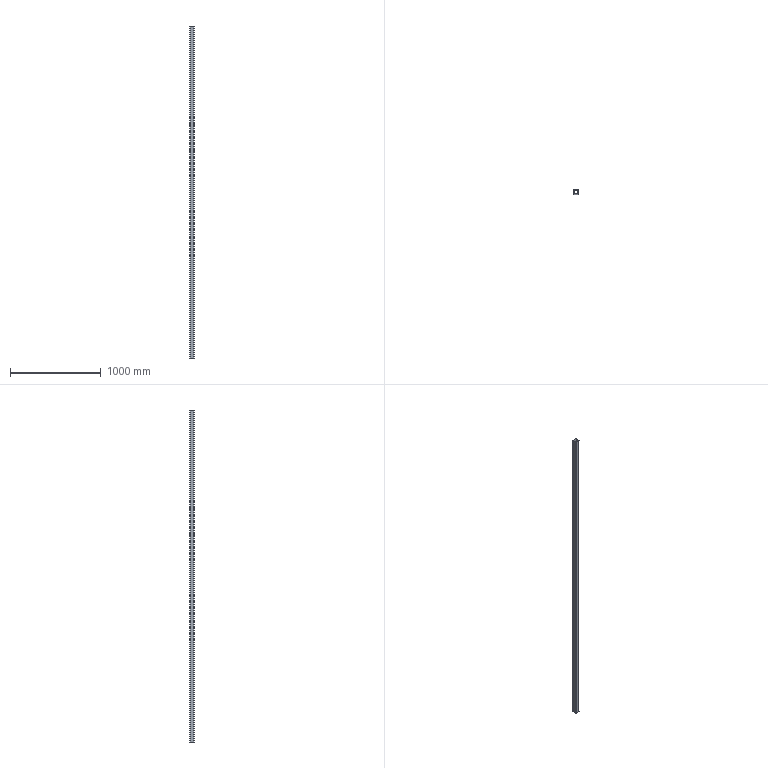Part | STEP file | Square steel 50×50×3650 | 1 solid | 18 faces | box 50 x 50 x 3650 mm | volume 2611204 mm3 | plane 10 | cylinder 8 | commonest cylinder face diameters 2 x4 10 x4
STEP:
#1=CARTESIAN_POINT('',(0.,0.,0.));
#2=DIRECTION('',(0.,0.,1.));
#3=DIRECTION('',(1.,0.,0.));
#4=AXIS2_PLACEMENT_3D('',#1,#2,#3);
#5=CARTESIAN_POINT('',(-25.,-20.,1825.));
#6=VERTEX_POINT('',#5);
#7=CARTESIAN_POINT('',(-20.,-25.,1825.));
#8=VERTEX_POINT('',#7);
#9=CARTESIAN_POINT('',(-20.,-20.,1825.));
#10=DIRECTION('',(0.,0.,1.));
#11=DIRECTION('',(1.,0.,0.));
#12=AXIS2_PLACEMENT_3D('',#9,#10,#11);
#13=CIRCLE('',#12,5.);
#14=CARTESIAN_POINT('',(-20.,-20.,1825.));
#15=DIRECTION('',(0.,0.,1.));
#16=DIRECTION('',(1.,0.,0.));
#17=AXIS2_PLACEMENT_3D('',#14,#15,#16);
#18=PLANE('',#17);
#19=CARTESIAN_POINT('',(0.,0.));
#20=DIRECTION('',(1.,0.));
#21=AXIS2_PLACEMENT_2D('',#19,#20);
#22=CIRCLE('',#21,5.);
#23=(GEOMETRIC_REPRESENTATION_CONTEXT(2)PARAMETRIC_REPRESENTATION_CONTEXT()REPRESENTATION_CONTEXT('',''));
#24=DEFINITIONAL_REPRESENTATION('',(#22),#23);
#25=PCURVE('',#18,#24);
#26=CARTESIAN_POINT('',(-20.,-20.,1825.));
#27=DIRECTION('',(0.,0.,-1.));
#28=DIRECTION('',(-1.,0.,0.));
#29=AXIS2_PLACEMENT_3D('',#26,#27,#28);
#30=CYLINDRICAL_SURFACE('',#29,5.);
#31=CARTESIAN_POINT('',(9.425,0.));
#32=DIRECTION('',(-1.,0.));
#33=VECTOR('',#32,1.);
#34=LINE('',#31,#33);
#35=(GEOMETRIC_REPRESENTATION_CONTEXT(2)PARAMETRIC_REPRESENTATION_CONTEXT()REPRESENTATION_CONTEXT('',''));
#36=DEFINITIONAL_REPRESENTATION('',(#34),#35);
#37=PCURVE('',#30,#36);
#38=SURFACE_CURVE('',#13,(#25,#37),.PCURVE_S1.);
#39=EDGE_CURVE('',#6,#8,#38,.T.);
#40=ORIENTED_EDGE('',*,*,#39,.T.);
#41=CARTESIAN_POINT('',(20.,-25.,1825.));
#42=VERTEX_POINT('',#41);
#43=CARTESIAN_POINT('',(-20.,-25.,1825.));
#44=DIRECTION('',(1.,0.,0.));
#45=VECTOR('',#44,1.);
#46=LINE('',#43,#45);
#47=CARTESIAN_POINT('',(0.,-5.));
#48=DIRECTION('',(1.,0.));
#49=VECTOR('',#48,1.);
#50=LINE('',#47,#49);
#51=(GEOMETRIC_REPRESENTATION_CONTEXT(2)PARAMETRIC_REPRESENTATION_CONTEXT()REPRESENTATION_CONTEXT('',''));
#52=DEFINITIONAL_REPRESENTATION('',(#50),#51);
#53=PCURVE('',#18,#52);
#54=CARTESIAN_POINT('',(-20.,-25.,1825.));
#55=DIRECTION('',(0.,1.,0.));
#56=DIRECTION('',(0.,0.,1.));
#57=AXIS2_PLACEMENT_3D('',#54,#55,#56);
#58=PLANE('',#57);
#59=CARTESIAN_POINT('',(0.,0.));
#60=DIRECTION('',(0.,1.));
#61=VECTOR('',#60,1.);
#62=LINE('',#59,#61);
#63=(GEOMETRIC_REPRESENTATION_CONTEXT(2)PARAMETRIC_REPRESENTATION_CONTEXT()REPRESENTATION_CONTEXT('',''));
#64=DEFINITIONAL_REPRESENTATION('',(#62),#63);
#65=PCURVE('',#58,#64);
#66=SURFACE_CURVE('',#46,(#53,#65),.PCURVE_S1.);
#67=EDGE_CURVE('',#8,#42,#66,.T.);
#68=ORIENTED_EDGE('',*,*,#67,.T.);
#69=CARTESIAN_POINT('',(25.,-20.,1825.));
#70=VERTEX_POINT('',#69);
#71=CARTESIAN_POINT('',(20.,-20.,1825.));
#72=DIRECTION('',(0.,0.,1.));
#73=DIRECTION('',(-1.,0.,0.));
#74=AXIS2_PLACEMENT_3D('',#71,#72,#73);
#75=CIRCLE('',#74,5.);
#76=CARTESIAN_POINT('',(40.,0.));
#77=DIRECTION('',(-1.,0.));
#78=AXIS2_PLACEMENT_2D('',#76,#77);
#79=CIRCLE('',#78,5.);
#80=(GEOMETRIC_REPRESENTATION_CONTEXT(2)PARAMETRIC_REPRESENTATION_CONTEXT()REPRESENTATION_CONTEXT('',''));
#81=DEFINITIONAL_REPRESENTATION('',(#79),#80);
#82=PCURVE('',#18,#81);
#83=CARTESIAN_POINT('',(20.,-20.,1825.));
#84=DIRECTION('',(0.,0.,-1.));
#85=DIRECTION('',(-1.,0.,0.));
#86=AXIS2_PLACEMENT_3D('',#83,#84,#85);
#87=CYLINDRICAL_SURFACE('',#86,5.);
#88=CARTESIAN_POINT('',(6.283,0.));
#89=DIRECTION('',(-1.,0.));
#90=VECTOR('',#89,1.);
#91=LINE('',#88,#90);
#92=(GEOMETRIC_REPRESENTATION_CONTEXT(2)PARAMETRIC_REPRESENTATION_CONTEXT()REPRESENTATION_CONTEXT('',''));
#93=DEFINITIONAL_REPRESENTATION('',(#91),#92);
#94=PCURVE('',#87,#93);
#95=SURFACE_CURVE('',#75,(#82,#94),.PCURVE_S1.);
#96=EDGE_CURVE('',#42,#70,#95,.T.);
#97=ORIENTED_EDGE('',*,*,#96,.T.);
#98=CARTESIAN_POINT('',(25.,20.,1825.));
#99=VERTEX_POINT('',#98);
#100=CARTESIAN_POINT('',(25.,20.,1825.));
#101=DIRECTION('',(0.,1.,0.));
#102=VECTOR('',#101,1.);
#103=LINE('',#100,#102);
#104=CARTESIAN_POINT('',(45.,40.));
#105=DIRECTION('',(0.,1.));
#106=VECTOR('',#105,1.);
#107=LINE('',#104,#106);
#108=(GEOMETRIC_REPRESENTATION_CONTEXT(2)PARAMETRIC_REPRESENTATION_CONTEXT()REPRESENTATION_CONTEXT('',''));
#109=DEFINITIONAL_REPRESENTATION('',(#107),#108);
#110=PCURVE('',#18,#109);
#111=CARTESIAN_POINT('',(25.,20.,1825.));
#112=DIRECTION('',(-1.,0.,0.));
#113=DIRECTION('',(0.,-1.,0.));
#114=AXIS2_PLACEMENT_3D('',#111,#112,#113);
#115=PLANE('',#114);
#116=CARTESIAN_POINT('',(0.,0.));
#117=DIRECTION('',(-1.,0.));
#118=VECTOR('',#117,1.);
#119=LINE('',#116,#118);
#120=(GEOMETRIC_REPRESENTATION_CONTEXT(2)PARAMETRIC_REPRESENTATION_CONTEXT()REPRESENTATION_CONTEXT('',''));
#121=DEFINITIONAL_REPRESENTATION('',(#119),#120);
#122=PCURVE('',#115,#121);
#123=SURFACE_CURVE('',#103,(#110,#122),.PCURVE_S1.);
#124=EDGE_CURVE('',#70,#99,#123,.T.);
#125=ORIENTED_EDGE('',*,*,#124,.T.);
#126=CARTESIAN_POINT('',(20.,25.,1825.));
#127=VERTEX_POINT('',#126);
#128=CARTESIAN_POINT('',(20.,20.,1825.));
#129=DIRECTION('',(0.,0.,1.));
#130=DIRECTION('',(1.,0.,0.));
#131=AXIS2_PLACEMENT_3D('',#128,#129,#130);
#132=CIRCLE('',#131,5.);
#133=CARTESIAN_POINT('',(40.,40.));
#134=DIRECTION('',(1.,0.));
#135=AXIS2_PLACEMENT_2D('',#133,#134);
#136=CIRCLE('',#135,5.);
#137=(GEOMETRIC_REPRESENTATION_CONTEXT(2)PARAMETRIC_REPRESENTATION_CONTEXT()REPRESENTATION_CONTEXT('',''));
#138=DEFINITIONAL_REPRESENTATION('',(#136),#137);
#139=PCURVE('',#18,#138);
#140=CARTESIAN_POINT('',(20.,20.,1825.));
#141=DIRECTION('',(0.,0.,-1.));
#142=DIRECTION('',(-1.,0.,0.));
#143=AXIS2_PLACEMENT_3D('',#140,#141,#142);
#144=CYLINDRICAL_SURFACE('',#143,5.);
#145=CARTESIAN_POINT('',(3.142,0.));
#146=DIRECTION('',(-1.,0.));
#147=VECTOR('',#146,1.);
#148=LINE('',#145,#147);
#149=(GEOMETRIC_REPRESENTATION_CONTEXT(2)PARAMETRIC_REPRESENTATION_CONTEXT()REPRESENTATION_CONTEXT('',''));
#150=DEFINITIONAL_REPRESENTATION('',(#148),#149);
#151=PCURVE('',#144,#150);
#152=SURFACE_CURVE('',#132,(#139,#151),.PCURVE_S1.);
#153=EDGE_CURVE('',#99,#127,#152,.T.);
#154=ORIENTED_EDGE('',*,*,#153,.T.);
#155=CARTESIAN_POINT('',(-20.,25.,1825.));
#156=VERTEX_POINT('',#155);
#157=CARTESIAN_POINT('',(-20.,25.,1825.));
#158=DIRECTION('',(-1.,0.,0.));
#159=VECTOR('',#158,1.);
#160=LINE('',#157,#159);
#161=CARTESIAN_POINT('',(0.,45.));
#162=DIRECTION('',(-1.,0.));
#163=VECTOR('',#162,1.);
#164=LINE('',#161,#163);
#165=(GEOMETRIC_REPRESENTATION_CONTEXT(2)PARAMETRIC_REPRESENTATION_CONTEXT()REPRESENTATION_CONTEXT('',''));
#166=DEFINITIONAL_REPRESENTATION('',(#164),#165);
#167=PCURVE('',#18,#166);
#168=CARTESIAN_POINT('',(-20.,25.,1825.));
#169=DIRECTION('',(0.,-1.,0.));
#170=DIRECTION('',(0.,0.,-1.));
#171=AXIS2_PLACEMENT_3D('',#168,#169,#170);
#172=PLANE('',#171);
#173=CARTESIAN_POINT('',(0.,0.));
#174=DIRECTION('',(0.,-1.));
#175=VECTOR('',#174,1.);
#176=LINE('',#173,#175);
#177=(GEOMETRIC_REPRESENTATION_CONTEXT(2)PARAMETRIC_REPRESENTATION_CONTEXT()REPRESENTATION_CONTEXT('',''));
#178=DEFINITIONAL_REPRESENTATION('',(#176),#177);
#179=PCURVE('',#172,#178);
#180=SURFACE_CURVE('',#160,(#167,#179),.PCURVE_S1.);
#181=EDGE_CURVE('',#127,#156,#180,.T.);
#182=ORIENTED_EDGE('',*,*,#181,.T.);
#183=CARTESIAN_POINT('',(-25.,20.,1825.));
#184=VERTEX_POINT('',#183);
#185=CARTESIAN_POINT('',(-20.,20.,1825.));
#186=DIRECTION('',(0.,0.,1.));
#187=DIRECTION('',(-1.,0.,0.));
#188=AXIS2_PLACEMENT_3D('',#185,#186,#187);
#189=CIRCLE('',#188,5.);
#190=CARTESIAN_POINT('',(0.,40.));
#191=DIRECTION('',(-1.,0.));
#192=AXIS2_PLACEMENT_2D('',#190,#191);
#193=CIRCLE('',#192,5.);
#194=(GEOMETRIC_REPRESENTATION_CONTEXT(2)PARAMETRIC_REPRESENTATION_CONTEXT()REPRESENTATION_CONTEXT('',''));
#195=DEFINITIONAL_REPRESENTATION('',(#193),#194);
#196=PCURVE('',#18,#195);
#197=CARTESIAN_POINT('',(-20.,20.,1825.));
#198=DIRECTION('',(0.,0.,-1.));
#199=DIRECTION('',(-1.,0.,0.));
#200=AXIS2_PLACEMENT_3D('',#197,#198,#199);
#201=CYLINDRICAL_SURFACE('',#200,5.);
#202=CARTESIAN_POINT('',(6.283,0.));
#203=DIRECTION('',(-1.,0.));
#204=VECTOR('',#203,1.);
#205=LINE('',#202,#204);
#206=(GEOMETRIC_REPRESENTATION_CONTEXT(2)PARAMETRIC_REPRESENTATION_CONTEXT()REPRESENTATION_CONTEXT('',''));
#207=DEFINITIONAL_REPRESENTATION('',(#205),#206);
#208=PCURVE('',#201,#207);
#209=SURFACE_CURVE('',#189,(#196,#208),.PCURVE_S1.);
#210=EDGE_CURVE('',#156,#184,#209,.T.);
#211=ORIENTED_EDGE('',*,*,#210,.T.);
#212=CARTESIAN_POINT('',(-25.,20.,1825.));
#213=DIRECTION('',(0.,-1.,0.));
#214=VECTOR('',#213,1.);
#215=LINE('',#212,#214);
#216=CARTESIAN_POINT('',(-5.,40.));
#217=DIRECTION('',(0.,-1.));
#218=VECTOR('',#217,1.);
#219=LINE('',#216,#218);
#220=(GEOMETRIC_REPRESENTATION_CONTEXT(2)PARAMETRIC_REPRESENTATION_CONTEXT()REPRESENTATION_CONTEXT('',''));
#221=DEFINITIONAL_REPRESENTATION('',(#219),#220);
#222=PCURVE('',#18,#221);
#223=CARTESIAN_POINT('',(-25.,20.,1825.));
#224=DIRECTION('',(1.,0.,0.));
#225=DIRECTION('',(0.,1.,0.));
#226=AXIS2_PLACEMENT_3D('',#223,#224,#225);
#227=PLANE('',#226);
#228=CARTESIAN_POINT('',(0.,0.));
#229=DIRECTION('',(-1.,0.));
#230=VECTOR('',#229,1.);
#231=LINE('',#228,#230);
#232=(GEOMETRIC_REPRESENTATION_CONTEXT(2)PARAMETRIC_REPRESENTATION_CONTEXT()REPRESENTATION_CONTEXT('',''));
#233=DEFINITIONAL_REPRESENTATION('',(#231),#232);
#234=PCURVE('',#227,#233);
#235=SURFACE_CURVE('',#215,(#222,#234),.PCURVE_S1.);
#236=EDGE_CURVE('',#184,#6,#235,.T.);
#237=ORIENTED_EDGE('',*,*,#236,.T.);
#238=EDGE_LOOP('',(#40,#68,#97,#125,#154,#182,#211,#237));
#239=FACE_BOUND('',#238,.T.);
#240=CARTESIAN_POINT('',(-21.,20.,1825.));
#241=VERTEX_POINT('',#240);
#242=CARTESIAN_POINT('',(-21.,-20.,1825.));
#243=VERTEX_POINT('',#242);
#244=CARTESIAN_POINT('',(-21.,20.,1825.));
#245=DIRECTION('',(0.,-1.,0.));
#246=VECTOR('',#245,1.);
#247=LINE('',#244,#246);
#248=CARTESIAN_POINT('',(-1.,40.));
#249=DIRECTION('',(0.,-1.));
#250=VECTOR('',#249,1.);
#251=LINE('',#248,#250);
#252=(GEOMETRIC_REPRESENTATION_CONTEXT(2)PARAMETRIC_REPRESENTATION_CONTEXT()REPRESENTATION_CONTEXT('',''));
#253=DEFINITIONAL_REPRESENTATION('',(#251),#252);
#254=PCURVE('',#18,#253);
#255=CARTESIAN_POINT('',(-21.,20.,1825.));
#256=DIRECTION('',(1.,0.,0.));
#257=DIRECTION('',(0.,1.,0.));
#258=AXIS2_PLACEMENT_3D('',#255,#256,#257);
#259=PLANE('',#258);
#260=CARTESIAN_POINT('',(0.,0.));
#261=DIRECTION('',(-1.,0.));
#262=VECTOR('',#261,1.);
#263=LINE('',#260,#262);
#264=(GEOMETRIC_REPRESENTATION_CONTEXT(2)PARAMETRIC_REPRESENTATION_CONTEXT()REPRESENTATION_CONTEXT('',''));
#265=DEFINITIONAL_REPRESENTATION('',(#263),#264);
#266=PCURVE('',#259,#265);
#267=SURFACE_CURVE('',#247,(#254,#266),.PCURVE_S1.);
#268=EDGE_CURVE('',#241,#243,#267,.T.);
#269=ORIENTED_EDGE('',*,*,#268,.F.);
#270=CARTESIAN_POINT('',(-20.,21.,1825.));
#271=VERTEX_POINT('',#270);
#272=CARTESIAN_POINT('',(-20.,20.,1825.));
#273=DIRECTION('',(0.,0.,1.));
#274=DIRECTION('',(-1.,0.,0.));
#275=AXIS2_PLACEMENT_3D('',#272,#273,#274);
#276=CIRCLE('',#275,1.);
#277=CARTESIAN_POINT('',(0.,40.));
#278=DIRECTION('',(-1.,0.));
#279=AXIS2_PLACEMENT_2D('',#277,#278);
#280=CIRCLE('',#279,1.);
#281=(GEOMETRIC_REPRESENTATION_CONTEXT(2)PARAMETRIC_REPRESENTATION_CONTEXT()REPRESENTATION_CONTEXT('',''));
#282=DEFINITIONAL_REPRESENTATION('',(#280),#281);
#283=PCURVE('',#18,#282);
#284=CARTESIAN_POINT('',(-20.,20.,1825.));
#285=DIRECTION('',(0.,0.,-1.));
#286=DIRECTION('',(-1.,0.,0.));
#287=AXIS2_PLACEMENT_3D('',#284,#285,#286);
#288=CYLINDRICAL_SURFACE('',#287,1.);
#289=CARTESIAN_POINT('',(6.283,0.));
#290=DIRECTION('',(-1.,0.));
#291=VECTOR('',#290,1.);
#292=LINE('',#289,#291);
#293=(GEOMETRIC_REPRESENTATION_CONTEXT(2)PARAMETRIC_REPRESENTATION_CONTEXT()REPRESENTATION_CONTEXT('',''));
#294=DEFINITIONAL_REPRESENTATION('',(#292),#293);
#295=PCURVE('',#288,#294);
#296=SURFACE_CURVE('',#276,(#283,#295),.PCURVE_S1.);
#297=EDGE_CURVE('',#271,#241,#296,.T.);
#298=ORIENTED_EDGE('',*,*,#297,.F.);
#299=CARTESIAN_POINT('',(20.,21.,1825.));
#300=VERTEX_POINT('',#299);
#301=CARTESIAN_POINT('',(-20.,21.,1825.));
#302=DIRECTION('',(-1.,0.,0.));
#303=VECTOR('',#302,1.);
#304=LINE('',#301,#303);
#305=CARTESIAN_POINT('',(0.,41.));
#306=DIRECTION('',(-1.,0.));
#307=VECTOR('',#306,1.);
#308=LINE('',#305,#307);
#309=(GEOMETRIC_REPRESENTATION_CONTEXT(2)PARAMETRIC_REPRESENTATION_CONTEXT()REPRESENTATION_CONTEXT('',''));
#310=DEFINITIONAL_REPRESENTATION('',(#308),#309);
#311=PCURVE('',#18,#310);
#312=CARTESIAN_POINT('',(-20.,21.,1825.));
#313=DIRECTION('',(0.,-1.,0.));
#314=DIRECTION('',(0.,0.,-1.));
#315=AXIS2_PLACEMENT_3D('',#312,#313,#314);
#316=PLANE('',#315);
#317=CARTESIAN_POINT('',(0.,0.));
#318=DIRECTION('',(0.,-1.));
#319=VECTOR('',#318,1.);
#320=LINE('',#317,#319);
#321=(GEOMETRIC_REPRESENTATION_CONTEXT(2)PARAMETRIC_REPRESENTATION_CONTEXT()REPRESENTATION_CONTEXT('',''));
#322=DEFINITIONAL_REPRESENTATION('',(#320),#321);
#323=PCURVE('',#316,#322);
#324=SURFACE_CURVE('',#304,(#311,#323),.PCURVE_S1.);
#325=EDGE_CURVE('',#300,#271,#324,.T.);
#326=ORIENTED_EDGE('',*,*,#325,.F.);
#327=CARTESIAN_POINT('',(21.,20.,1825.));
#328=VERTEX_POINT('',#327);
#329=CARTESIAN_POINT('',(20.,20.,1825.));
#330=DIRECTION('',(0.,0.,1.));
#331=DIRECTION('',(1.,0.,0.));
#332=AXIS2_PLACEMENT_3D('',#329,#330,#331);
#333=CIRCLE('',#332,1.);
#334=CARTESIAN_POINT('',(40.,40.));
#335=DIRECTION('',(1.,0.));
#336=AXIS2_PLACEMENT_2D('',#334,#335);
#337=CIRCLE('',#336,1.);
#338=(GEOMETRIC_REPRESENTATION_CONTEXT(2)PARAMETRIC_REPRESENTATION_CONTEXT()REPRESENTATION_CONTEXT('',''));
#339=DEFINITIONAL_REPRESENTATION('',(#337),#338);
#340=PCURVE('',#18,#339);
#341=CARTESIAN_POINT('',(20.,20.,1825.));
#342=DIRECTION('',(0.,0.,-1.));
#343=DIRECTION('',(-1.,0.,0.));
#344=AXIS2_PLACEMENT_3D('',#341,#342,#343);
#345=CYLINDRICAL_SURFACE('',#344,1.);
#346=CARTESIAN_POINT('',(3.142,0.));
#347=DIRECTION('',(-1.,0.));
#348=VECTOR('',#347,1.);
#349=LINE('',#346,#348);
#350=(GEOMETRIC_REPRESENTATION_CONTEXT(2)PARAMETRIC_REPRESENTATION_CONTEXT()REPRESENTATION_CONTEXT('',''));
#351=DEFINITIONAL_REPRESENTATION('',(#349),#350);
#352=PCURVE('',#345,#351);
#353=SURFACE_CURVE('',#333,(#340,#352),.PCURVE_S1.);
#354=EDGE_CURVE('',#328,#300,#353,.T.);
#355=ORIENTED_EDGE('',*,*,#354,.F.);
#356=CARTESIAN_POINT('',(21.,-20.,1825.));
#357=VERTEX_POINT('',#356);
#358=CARTESIAN_POINT('',(21.,20.,1825.));
#359=DIRECTION('',(0.,1.,0.));
#360=VECTOR('',#359,1.);
#361=LINE('',#358,#360);
#362=CARTESIAN_POINT('',(41.,40.));
#363=DIRECTION('',(0.,1.));
#364=VECTOR('',#363,1.);
#365=LINE('',#362,#364);
#366=(GEOMETRIC_REPRESENTATION_CONTEXT(2)PARAMETRIC_REPRESENTATION_CONTEXT()REPRESENTATION_CONTEXT('',''));
#367=DEFINITIONAL_REPRESENTATION('',(#365),#366);
#368=PCURVE('',#18,#367);
#369=CARTESIAN_POINT('',(21.,20.,1825.));
#370=DIRECTION('',(-1.,0.,0.));
#371=DIRECTION('',(0.,0.,1.));
#372=AXIS2_PLACEMENT_3D('',#369,#370,#371);
#373=PLANE('',#372);
#374=CARTESIAN_POINT('',(0.,0.));
#375=DIRECTION('',(0.,1.));
#376=VECTOR('',#375,1.);
#377=LINE('',#374,#376);
#378=(GEOMETRIC_REPRESENTATION_CONTEXT(2)PARAMETRIC_REPRESENTATION_CONTEXT()REPRESENTATION_CONTEXT('',''));
#379=DEFINITIONAL_REPRESENTATION('',(#377),#378);
#380=PCURVE('',#373,#379);
#381=SURFACE_CURVE('',#361,(#368,#380),.PCURVE_S1.);
#382=EDGE_CURVE('',#357,#328,#381,.T.);
#383=ORIENTED_EDGE('',*,*,#382,.F.);
#384=CARTESIAN_POINT('',(20.,-21.,1825.));
#385=VERTEX_POINT('',#384);
#386=CARTESIAN_POINT('',(20.,-20.,1825.));
#387=DIRECTION('',(0.,0.,1.));
#388=DIRECTION('',(-1.,0.,0.));
#389=AXIS2_PLACEMENT_3D('',#386,#387,#388);
#390=CIRCLE('',#389,1.);
#391=CARTESIAN_POINT('',(40.,0.));
#392=DIRECTION('',(-1.,0.));
#393=AXIS2_PLACEMENT_2D('',#391,#392);
#394=CIRCLE('',#393,1.);
#395=(GEOMETRIC_REPRESENTATION_CONTEXT(2)PARAMETRIC_REPRESENTATION_CONTEXT()REPRESENTATION_CONTEXT('',''));
#396=DEFINITIONAL_REPRESENTATION('',(#394),#395);
#397=PCURVE('',#18,#396);
#398=CARTESIAN_POINT('',(20.,-20.,1825.));
#399=DIRECTION('',(0.,0.,-1.));
#400=DIRECTION('',(-1.,0.,0.));
#401=AXIS2_PLACEMENT_3D('',#398,#399,#400);
#402=CYLINDRICAL_SURFACE('',#401,1.);
#403=CARTESIAN_POINT('',(6.283,0.));
#404=DIRECTION('',(-1.,0.));
#405=VECTOR('',#404,1.);
#406=LINE('',#403,#405);
#407=(GEOMETRIC_REPRESENTATION_CONTEXT(2)PARAMETRIC_REPRESENTATION_CONTEXT()REPRESENTATION_CONTEXT('',''));
#408=DEFINITIONAL_REPRESENTATION('',(#406),#407);
#409=PCURVE('',#402,#408);
#410=SURFACE_CURVE('',#390,(#397,#409),.PCURVE_S1.);
#411=EDGE_CURVE('',#385,#357,#410,.T.);
#412=ORIENTED_EDGE('',*,*,#411,.F.);
#413=CARTESIAN_POINT('',(-20.,-21.,1825.));
#414=VERTEX_POINT('',#413);
#415=CARTESIAN_POINT('',(-20.,-21.,1825.));
#416=DIRECTION('',(1.,0.,0.));
#417=VECTOR('',#416,1.);
#418=LINE('',#415,#417);
#419=CARTESIAN_POINT('',(0.,-1.));
#420=DIRECTION('',(1.,0.));
#421=VECTOR('',#420,1.);
#422=LINE('',#419,#421);
#423=(GEOMETRIC_REPRESENTATION_CONTEXT(2)PARAMETRIC_REPRESENTATION_CONTEXT()REPRESENTATION_CONTEXT('',''));
#424=DEFINITIONAL_REPRESENTATION('',(#422),#423);
#425=PCURVE('',#18,#424);
#426=CARTESIAN_POINT('',(-20.,-21.,1825.));
#427=DIRECTION('',(0.,1.,0.));
#428=DIRECTION('',(0.,0.,1.));
#429=AXIS2_PLACEMENT_3D('',#426,#427,#428);
#430=PLANE('',#429);
#431=CARTESIAN_POINT('',(0.,0.));
#432=DIRECTION('',(0.,1.));
#433=VECTOR('',#432,1.);
#434=LINE('',#431,#433);
#435=(GEOMETRIC_REPRESENTATION_CONTEXT(2)PARAMETRIC_REPRESENTATION_CONTEXT()REPRESENTATION_CONTEXT('',''));
#436=DEFINITIONAL_REPRESENTATION('',(#434),#435);
#437=PCURVE('',#430,#436);
#438=SURFACE_CURVE('',#418,(#425,#437),.PCURVE_S1.);
#439=EDGE_CURVE('',#414,#385,#438,.T.);
#440=ORIENTED_EDGE('',*,*,#439,.F.);
#441=CARTESIAN_POINT('',(-20.,-20.,1825.));
#442=DIRECTION('',(0.,0.,1.));
#443=DIRECTION('',(1.,0.,0.));
#444=AXIS2_PLACEMENT_3D('',#441,#442,#443);
#445=CIRCLE('',#444,1.);
#446=CARTESIAN_POINT('',(0.,0.));
#447=DIRECTION('',(1.,0.));
#448=AXIS2_PLACEMENT_2D('',#446,#447);
#449=CIRCLE('',#448,1.);
#450=(GEOMETRIC_REPRESENTATION_CONTEXT(2)PARAMETRIC_REPRESENTATION_CONTEXT()REPRESENTATION_CONTEXT('',''));
#451=DEFINITIONAL_REPRESENTATION('',(#449),#450);
#452=PCURVE('',#18,#451);
#453=CARTESIAN_POINT('',(-20.,-20.,1825.));
#454=DIRECTION('',(0.,0.,-1.));
#455=DIRECTION('',(-1.,0.,0.));
#456=AXIS2_PLACEMENT_3D('',#453,#454,#455);
#457=CYLINDRICAL_SURFACE('',#456,1.);
#458=CARTESIAN_POINT('',(9.425,0.));
#459=DIRECTION('',(-1.,0.));
#460=VECTOR('',#459,1.);
#461=LINE('',#458,#460);
#462=(GEOMETRIC_REPRESENTATION_CONTEXT(2)PARAMETRIC_REPRESENTATION_CONTEXT()REPRESENTATION_CONTEXT('',''));
#463=DEFINITIONAL_REPRESENTATION('',(#461),#462);
#464=PCURVE('',#457,#463);
#465=SURFACE_CURVE('',#445,(#452,#464),.PCURVE_S1.);
#466=EDGE_CURVE('',#243,#414,#465,.T.);
#467=ORIENTED_EDGE('',*,*,#466,.F.);
#468=EDGE_LOOP('',(#269,#298,#326,#355,#383,#412,#440,#467));
#469=FACE_BOUND('',#468,.T.);
#470=ADVANCED_FACE('',(#239,#469),#18,.T.);
#471=CARTESIAN_POINT('',(-25.,-20.,-1825.));
#472=VERTEX_POINT('',#471);
#473=CARTESIAN_POINT('',(-20.,-25.,-1825.));
#474=VERTEX_POINT('',#473);
#475=CARTESIAN_POINT('',(-20.,-20.,-1825.));
#476=DIRECTION('',(0.,0.,1.));
#477=DIRECTION('',(1.,0.,0.));
#478=AXIS2_PLACEMENT_3D('',#475,#476,#477);
#479=CIRCLE('',#478,5.);
#480=CARTESIAN_POINT('',(-20.,-20.,-1825.));
#481=DIRECTION('',(0.,0.,1.));
#482=DIRECTION('',(1.,0.,0.));
#483=AXIS2_PLACEMENT_3D('',#480,#481,#482);
#484=PLANE('',#483);
#485=CARTESIAN_POINT('',(0.,0.));
#486=DIRECTION('',(1.,0.));
#487=AXIS2_PLACEMENT_2D('',#485,#486);
#488=CIRCLE('',#487,5.);
#489=(GEOMETRIC_REPRESENTATION_CONTEXT(2)PARAMETRIC_REPRESENTATION_CONTEXT()REPRESENTATION_CONTEXT('',''));
#490=DEFINITIONAL_REPRESENTATION('',(#488),#489);
#491=PCURVE('',#484,#490);
#492=CARTESIAN_POINT('',(9.425,3650.));
#493=DIRECTION('',(-1.,0.));
#494=VECTOR('',#493,1.);
#495=LINE('',#492,#494);
#496=(GEOMETRIC_REPRESENTATION_CONTEXT(2)PARAMETRIC_REPRESENTATION_CONTEXT()REPRESENTATION_CONTEXT('',''));
#497=DEFINITIONAL_REPRESENTATION('',(#495),#496);
#498=PCURVE('',#30,#497);
#499=SURFACE_CURVE('',#479,(#491,#498),.PCURVE_S1.);
#500=EDGE_CURVE('',#472,#474,#499,.T.);
#501=ORIENTED_EDGE('',*,*,#500,.F.);
#502=CARTESIAN_POINT('',(-25.,20.,-1825.));
#503=VERTEX_POINT('',#502);
#504=CARTESIAN_POINT('',(-25.,20.,-1825.));
#505=DIRECTION('',(0.,-1.,0.));
#506=VECTOR('',#505,1.);
#507=LINE('',#504,#506);
#508=CARTESIAN_POINT('',(-5.,40.));
#509=DIRECTION('',(0.,-1.));
#510=VECTOR('',#509,1.);
#511=LINE('',#508,#510);
#512=(GEOMETRIC_REPRESENTATION_CONTEXT(2)PARAMETRIC_REPRESENTATION_CONTEXT()REPRESENTATION_CONTEXT('',''));
#513=DEFINITIONAL_REPRESENTATION('',(#511),#512);
#514=PCURVE('',#484,#513);
#515=CARTESIAN_POINT('',(0.,-3650.));
#516=DIRECTION('',(-1.,0.));
#517=VECTOR('',#516,1.);
#518=LINE('',#515,#517);
#519=(GEOMETRIC_REPRESENTATION_CONTEXT(2)PARAMETRIC_REPRESENTATION_CONTEXT()REPRESENTATION_CONTEXT('',''));
#520=DEFINITIONAL_REPRESENTATION('',(#518),#519);
#521=PCURVE('',#227,#520);
#522=SURFACE_CURVE('',#507,(#514,#521),.PCURVE_S1.);
#523=EDGE_CURVE('',#503,#472,#522,.T.);
#524=ORIENTED_EDGE('',*,*,#523,.F.);
#525=CARTESIAN_POINT('',(-20.,25.,-1825.));
#526=VERTEX_POINT('',#525);
#527=CARTESIAN_POINT('',(-20.,20.,-1825.));
#528=DIRECTION('',(0.,0.,1.));
#529=DIRECTION('',(-1.,0.,0.));
#530=AXIS2_PLACEMENT_3D('',#527,#528,#529);
#531=CIRCLE('',#530,5.);
#532=CARTESIAN_POINT('',(0.,40.));
#533=DIRECTION('',(-1.,0.));
#534=AXIS2_PLACEMENT_2D('',#532,#533);
#535=CIRCLE('',#534,5.);
#536=(GEOMETRIC_REPRESENTATION_CONTEXT(2)PARAMETRIC_REPRESENTATION_CONTEXT()REPRESENTATION_CONTEXT('',''));
#537=DEFINITIONAL_REPRESENTATION('',(#535),#536);
#538=PCURVE('',#484,#537);
#539=CARTESIAN_POINT('',(6.283,3650.));
#540=DIRECTION('',(-1.,0.));
#541=VECTOR('',#540,1.);
#542=LINE('',#539,#541);
#543=(GEOMETRIC_REPRESENTATION_CONTEXT(2)PARAMETRIC_REPRESENTATION_CONTEXT()REPRESENTATION_CONTEXT('',''));
#544=DEFINITIONAL_REPRESENTATION('',(#542),#543);
#545=PCURVE('',#201,#544);
#546=SURFACE_CURVE('',#531,(#538,#545),.PCURVE_S1.);
#547=EDGE_CURVE('',#526,#503,#546,.T.);
#548=ORIENTED_EDGE('',*,*,#547,.F.);
#549=CARTESIAN_POINT('',(20.,25.,-1825.));
#550=VERTEX_POINT('',#549);
#551=CARTESIAN_POINT('',(-20.,25.,-1825.));
#552=DIRECTION('',(-1.,0.,0.));
#553=VECTOR('',#552,1.);
#554=LINE('',#551,#553);
#555=CARTESIAN_POINT('',(0.,45.));
#556=DIRECTION('',(-1.,0.));
#557=VECTOR('',#556,1.);
#558=LINE('',#555,#557);
#559=(GEOMETRIC_REPRESENTATION_CONTEXT(2)PARAMETRIC_REPRESENTATION_CONTEXT()REPRESENTATION_CONTEXT('',''));
#560=DEFINITIONAL_REPRESENTATION('',(#558),#559);
#561=PCURVE('',#484,#560);
#562=CARTESIAN_POINT('',(3650.,0.));
#563=DIRECTION('',(0.,-1.));
#564=VECTOR('',#563,1.);
#565=LINE('',#562,#564);
#566=(GEOMETRIC_REPRESENTATION_CONTEXT(2)PARAMETRIC_REPRESENTATION_CONTEXT()REPRESENTATION_CONTEXT('',''));
#567=DEFINITIONAL_REPRESENTATION('',(#565),#566);
#568=PCURVE('',#172,#567);
#569=SURFACE_CURVE('',#554,(#561,#568),.PCURVE_S1.);
#570=EDGE_CURVE('',#550,#526,#569,.T.);
#571=ORIENTED_EDGE('',*,*,#570,.F.);
#572=CARTESIAN_POINT('',(25.,20.,-1825.));
#573=VERTEX_POINT('',#572);
#574=CARTESIAN_POINT('',(20.,20.,-1825.));
#575=DIRECTION('',(0.,0.,1.));
#576=DIRECTION('',(1.,0.,0.));
#577=AXIS2_PLACEMENT_3D('',#574,#575,#576);
#578=CIRCLE('',#577,5.);
#579=CARTESIAN_POINT('',(40.,40.));
#580=DIRECTION('',(1.,0.));
#581=AXIS2_PLACEMENT_2D('',#579,#580);
#582=CIRCLE('',#581,5.);
#583=(GEOMETRIC_REPRESENTATION_CONTEXT(2)PARAMETRIC_REPRESENTATION_CONTEXT()REPRESENTATION_CONTEXT('',''));
#584=DEFINITIONAL_REPRESENTATION('',(#582),#583);
#585=PCURVE('',#484,#584);
#586=CARTESIAN_POINT('',(3.142,3650.));
#587=DIRECTION('',(-1.,0.));
#588=VECTOR('',#587,1.);
#589=LINE('',#586,#588);
#590=(GEOMETRIC_REPRESENTATION_CONTEXT(2)PARAMETRIC_REPRESENTATION_CONTEXT()REPRESENTATION_CONTEXT('',''));
#591=DEFINITIONAL_REPRESENTATION('',(#589),#590);
#592=PCURVE('',#144,#591);
#593=SURFACE_CURVE('',#578,(#585,#592),.PCURVE_S1.);
#594=EDGE_CURVE('',#573,#550,#593,.T.);
#595=ORIENTED_EDGE('',*,*,#594,.F.);
#596=CARTESIAN_POINT('',(25.,-20.,-1825.));
#597=VERTEX_POINT('',#596);
#598=CARTESIAN_POINT('',(25.,20.,-1825.));
#599=DIRECTION('',(0.,1.,0.));
#600=VECTOR('',#599,1.);
#601=LINE('',#598,#600);
#602=CARTESIAN_POINT('',(45.,40.));
#603=DIRECTION('',(0.,1.));
#604=VECTOR('',#603,1.);
#605=LINE('',#602,#604);
#606=(GEOMETRIC_REPRESENTATION_CONTEXT(2)PARAMETRIC_REPRESENTATION_CONTEXT()REPRESENTATION_CONTEXT('',''));
#607=DEFINITIONAL_REPRESENTATION('',(#605),#606);
#608=PCURVE('',#484,#607);
#609=CARTESIAN_POINT('',(0.,-3650.));
#610=DIRECTION('',(-1.,0.));
#611=VECTOR('',#610,1.);
#612=LINE('',#609,#611);
#613=(GEOMETRIC_REPRESENTATION_CONTEXT(2)PARAMETRIC_REPRESENTATION_CONTEXT()REPRESENTATION_CONTEXT('',''));
#614=DEFINITIONAL_REPRESENTATION('',(#612),#613);
#615=PCURVE('',#115,#614);
#616=SURFACE_CURVE('',#601,(#608,#615),.PCURVE_S1.);
#617=EDGE_CURVE('',#597,#573,#616,.T.);
#618=ORIENTED_EDGE('',*,*,#617,.F.);
#619=CARTESIAN_POINT('',(20.,-25.,-1825.));
#620=VERTEX_POINT('',#619);
#621=CARTESIAN_POINT('',(20.,-20.,-1825.));
#622=DIRECTION('',(0.,0.,1.));
#623=DIRECTION('',(-1.,0.,0.));
#624=AXIS2_PLACEMENT_3D('',#621,#622,#623);
#625=CIRCLE('',#624,5.);
#626=CARTESIAN_POINT('',(40.,0.));
#627=DIRECTION('',(-1.,0.));
#628=AXIS2_PLACEMENT_2D('',#626,#627);
#629=CIRCLE('',#628,5.);
#630=(GEOMETRIC_REPRESENTATION_CONTEXT(2)PARAMETRIC_REPRESENTATION_CONTEXT()REPRESENTATION_CONTEXT('',''));
#631=DEFINITIONAL_REPRESENTATION('',(#629),#630);
#632=PCURVE('',#484,#631);
#633=CARTESIAN_POINT('',(6.283,3650.));
#634=DIRECTION('',(-1.,0.));
#635=VECTOR('',#634,1.);
#636=LINE('',#633,#635);
#637=(GEOMETRIC_REPRESENTATION_CONTEXT(2)PARAMETRIC_REPRESENTATION_CONTEXT()REPRESENTATION_CONTEXT('',''));
#638=DEFINITIONAL_REPRESENTATION('',(#636),#637);
#639=PCURVE('',#87,#638);
#640=SURFACE_CURVE('',#625,(#632,#639),.PCURVE_S1.);
#641=EDGE_CURVE('',#620,#597,#640,.T.);
#642=ORIENTED_EDGE('',*,*,#641,.F.);
#643=CARTESIAN_POINT('',(-20.,-25.,-1825.));
#644=DIRECTION('',(1.,0.,0.));
#645=VECTOR('',#644,1.);
#646=LINE('',#643,#645);
#647=CARTESIAN_POINT('',(0.,-5.));
#648=DIRECTION('',(1.,0.));
#649=VECTOR('',#648,1.);
#650=LINE('',#647,#649);
#651=(GEOMETRIC_REPRESENTATION_CONTEXT(2)PARAMETRIC_REPRESENTATION_CONTEXT()REPRESENTATION_CONTEXT('',''));
#652=DEFINITIONAL_REPRESENTATION('',(#650),#651);
#653=PCURVE('',#484,#652);
#654=CARTESIAN_POINT('',(-3650.,0.));
#655=DIRECTION('',(0.,1.));
#656=VECTOR('',#655,1.);
#657=LINE('',#654,#656);
#658=(GEOMETRIC_REPRESENTATION_CONTEXT(2)PARAMETRIC_REPRESENTATION_CONTEXT()REPRESENTATION_CONTEXT('',''));
#659=DEFINITIONAL_REPRESENTATION('',(#657),#658);
#660=PCURVE('',#58,#659);
#661=SURFACE_CURVE('',#646,(#653,#660),.PCURVE_S1.);
#662=EDGE_CURVE('',#474,#620,#661,.T.);
#663=ORIENTED_EDGE('',*,*,#662,.F.);
#664=EDGE_LOOP('',(#501,#524,#548,#571,#595,#618,#642,#663));
#665=FACE_BOUND('',#664,.T.);
#666=CARTESIAN_POINT('',(-20.,21.,-1825.));
#667=VERTEX_POINT('',#666);
#668=CARTESIAN_POINT('',(-21.,20.,-1825.));
#669=VERTEX_POINT('',#668);
#670=CARTESIAN_POINT('',(-20.,20.,-1825.));
#671=DIRECTION('',(0.,0.,1.));
#672=DIRECTION('',(-1.,0.,0.));
#673=AXIS2_PLACEMENT_3D('',#670,#671,#672);
#674=CIRCLE('',#673,1.);
#675=CARTESIAN_POINT('',(0.,40.));
#676=DIRECTION('',(-1.,0.));
#677=AXIS2_PLACEMENT_2D('',#675,#676);
#678=CIRCLE('',#677,1.);
#679=(GEOMETRIC_REPRESENTATION_CONTEXT(2)PARAMETRIC_REPRESENTATION_CONTEXT()REPRESENTATION_CONTEXT('',''));
#680=DEFINITIONAL_REPRESENTATION('',(#678),#679);
#681=PCURVE('',#484,#680);
#682=CARTESIAN_POINT('',(6.283,3650.));
#683=DIRECTION('',(-1.,0.));
#684=VECTOR('',#683,1.);
#685=LINE('',#682,#684);
#686=(GEOMETRIC_REPRESENTATION_CONTEXT(2)PARAMETRIC_REPRESENTATION_CONTEXT()REPRESENTATION_CONTEXT('',''));
#687=DEFINITIONAL_REPRESENTATION('',(#685),#686);
#688=PCURVE('',#288,#687);
#689=SURFACE_CURVE('',#674,(#681,#688),.PCURVE_S1.);
#690=EDGE_CURVE('',#667,#669,#689,.T.);
#691=ORIENTED_EDGE('',*,*,#690,.T.);
#692=CARTESIAN_POINT('',(-21.,-20.,-1825.));
#693=VERTEX_POINT('',#692);
#694=CARTESIAN_POINT('',(-21.,20.,-1825.));
#695=DIRECTION('',(0.,-1.,0.));
#696=VECTOR('',#695,1.);
#697=LINE('',#694,#696);
#698=CARTESIAN_POINT('',(-1.,40.));
#699=DIRECTION('',(0.,-1.));
#700=VECTOR('',#699,1.);
#701=LINE('',#698,#700);
#702=(GEOMETRIC_REPRESENTATION_CONTEXT(2)PARAMETRIC_REPRESENTATION_CONTEXT()REPRESENTATION_CONTEXT('',''));
#703=DEFINITIONAL_REPRESENTATION('',(#701),#702);
#704=PCURVE('',#484,#703);
#705=CARTESIAN_POINT('',(0.,-3650.));
#706=DIRECTION('',(-1.,0.));
#707=VECTOR('',#706,1.);
#708=LINE('',#705,#707);
#709=(GEOMETRIC_REPRESENTATION_CONTEXT(2)PARAMETRIC_REPRESENTATION_CONTEXT()REPRESENTATION_CONTEXT('',''));
#710=DEFINITIONAL_REPRESENTATION('',(#708),#709);
#711=PCURVE('',#259,#710);
#712=SURFACE_CURVE('',#697,(#704,#711),.PCURVE_S1.);
#713=EDGE_CURVE('',#669,#693,#712,.T.);
#714=ORIENTED_EDGE('',*,*,#713,.T.);
#715=CARTESIAN_POINT('',(-20.,-21.,-1825.));
#716=VERTEX_POINT('',#715);
#717=CARTESIAN_POINT('',(-20.,-20.,-1825.));
#718=DIRECTION('',(0.,0.,1.));
#719=DIRECTION('',(1.,0.,0.));
#720=AXIS2_PLACEMENT_3D('',#717,#718,#719);
#721=CIRCLE('',#720,1.);
#722=CARTESIAN_POINT('',(0.,0.));
#723=DIRECTION('',(1.,0.));
#724=AXIS2_PLACEMENT_2D('',#722,#723);
#725=CIRCLE('',#724,1.);
#726=(GEOMETRIC_REPRESENTATION_CONTEXT(2)PARAMETRIC_REPRESENTATION_CONTEXT()REPRESENTATION_CONTEXT('',''));
#727=DEFINITIONAL_REPRESENTATION('',(#725),#726);
#728=PCURVE('',#484,#727);
#729=CARTESIAN_POINT('',(9.425,3650.));
#730=DIRECTION('',(-1.,0.));
#731=VECTOR('',#730,1.);
#732=LINE('',#729,#731);
#733=(GEOMETRIC_REPRESENTATION_CONTEXT(2)PARAMETRIC_REPRESENTATION_CONTEXT()REPRESENTATION_CONTEXT('',''));
#734=DEFINITIONAL_REPRESENTATION('',(#732),#733);
#735=PCURVE('',#457,#734);
#736=SURFACE_CURVE('',#721,(#728,#735),.PCURVE_S1.);
#737=EDGE_CURVE('',#693,#716,#736,.T.);
#738=ORIENTED_EDGE('',*,*,#737,.T.);
#739=CARTESIAN_POINT('',(20.,-21.,-1825.));
#740=VERTEX_POINT('',#739);
#741=CARTESIAN_POINT('',(-20.,-21.,-1825.));
#742=DIRECTION('',(1.,0.,0.));
#743=VECTOR('',#742,1.);
#744=LINE('',#741,#743);
#745=CARTESIAN_POINT('',(0.,-1.));
#746=DIRECTION('',(1.,0.));
#747=VECTOR('',#746,1.);
#748=LINE('',#745,#747);
#749=(GEOMETRIC_REPRESENTATION_CONTEXT(2)PARAMETRIC_REPRESENTATION_CONTEXT()REPRESENTATION_CONTEXT('',''));
#750=DEFINITIONAL_REPRESENTATION('',(#748),#749);
#751=PCURVE('',#484,#750);
#752=CARTESIAN_POINT('',(-3650.,0.));
#753=DIRECTION('',(0.,1.));
#754=VECTOR('',#753,1.);
#755=LINE('',#752,#754);
#756=(GEOMETRIC_REPRESENTATION_CONTEXT(2)PARAMETRIC_REPRESENTATION_CONTEXT()REPRESENTATION_CONTEXT('',''));
#757=DEFINITIONAL_REPRESENTATION('',(#755),#756);
#758=PCURVE('',#430,#757);
#759=SURFACE_CURVE('',#744,(#751,#758),.PCURVE_S1.);
#760=EDGE_CURVE('',#716,#740,#759,.T.);
#761=ORIENTED_EDGE('',*,*,#760,.T.);
#762=CARTESIAN_POINT('',(21.,-20.,-1825.));
#763=VERTEX_POINT('',#762);
#764=CARTESIAN_POINT('',(20.,-20.,-1825.));
#765=DIRECTION('',(0.,0.,1.));
#766=DIRECTION('',(-1.,0.,0.));
#767=AXIS2_PLACEMENT_3D('',#764,#765,#766);
#768=CIRCLE('',#767,1.);
#769=CARTESIAN_POINT('',(40.,0.));
#770=DIRECTION('',(-1.,0.));
#771=AXIS2_PLACEMENT_2D('',#769,#770);
#772=CIRCLE('',#771,1.);
#773=(GEOMETRIC_REPRESENTATION_CONTEXT(2)PARAMETRIC_REPRESENTATION_CONTEXT()REPRESENTATION_CONTEXT('',''));
#774=DEFINITIONAL_REPRESENTATION('',(#772),#773);
#775=PCURVE('',#484,#774);
#776=CARTESIAN_POINT('',(6.283,3650.));
#777=DIRECTION('',(-1.,0.));
#778=VECTOR('',#777,1.);
#779=LINE('',#776,#778);
#780=(GEOMETRIC_REPRESENTATION_CONTEXT(2)PARAMETRIC_REPRESENTATION_CONTEXT()REPRESENTATION_CONTEXT('',''));
#781=DEFINITIONAL_REPRESENTATION('',(#779),#780);
#782=PCURVE('',#402,#781);
#783=SURFACE_CURVE('',#768,(#775,#782),.PCURVE_S1.);
#784=EDGE_CURVE('',#740,#763,#783,.T.);
#785=ORIENTED_EDGE('',*,*,#784,.T.);
#786=CARTESIAN_POINT('',(21.,20.,-1825.));
#787=VERTEX_POINT('',#786);
#788=CARTESIAN_POINT('',(21.,20.,-1825.));
#789=DIRECTION('',(0.,1.,0.));
#790=VECTOR('',#789,1.);
#791=LINE('',#788,#790);
#792=CARTESIAN_POINT('',(41.,40.));
#793=DIRECTION('',(0.,1.));
#794=VECTOR('',#793,1.);
#795=LINE('',#792,#794);
#796=(GEOMETRIC_REPRESENTATION_CONTEXT(2)PARAMETRIC_REPRESENTATION_CONTEXT()REPRESENTATION_CONTEXT('',''));
#797=DEFINITIONAL_REPRESENTATION('',(#795),#796);
#798=PCURVE('',#484,#797);
#799=CARTESIAN_POINT('',(-3650.,0.));
#800=DIRECTION('',(0.,1.));
#801=VECTOR('',#800,1.);
#802=LINE('',#799,#801);
#803=(GEOMETRIC_REPRESENTATION_CONTEXT(2)PARAMETRIC_REPRESENTATION_CONTEXT()REPRESENTATION_CONTEXT('',''));
#804=DEFINITIONAL_REPRESENTATION('',(#802),#803);
#805=PCURVE('',#373,#804);
#806=SURFACE_CURVE('',#791,(#798,#805),.PCURVE_S1.);
#807=EDGE_CURVE('',#763,#787,#806,.T.);
#808=ORIENTED_EDGE('',*,*,#807,.T.);
#809=CARTESIAN_POINT('',(20.,21.,-1825.));
#810=VERTEX_POINT('',#809);
#811=CARTESIAN_POINT('',(20.,20.,-1825.));
#812=DIRECTION('',(0.,0.,1.));
#813=DIRECTION('',(1.,0.,0.));
#814=AXIS2_PLACEMENT_3D('',#811,#812,#813);
#815=CIRCLE('',#814,1.);
#816=CARTESIAN_POINT('',(40.,40.));
#817=DIRECTION('',(1.,0.));
#818=AXIS2_PLACEMENT_2D('',#816,#817);
#819=CIRCLE('',#818,1.);
#820=(GEOMETRIC_REPRESENTATION_CONTEXT(2)PARAMETRIC_REPRESENTATION_CONTEXT()REPRESENTATION_CONTEXT('',''));
#821=DEFINITIONAL_REPRESENTATION('',(#819),#820);
#822=PCURVE('',#484,#821);
#823=CARTESIAN_POINT('',(3.142,3650.));
#824=DIRECTION('',(-1.,0.));
#825=VECTOR('',#824,1.);
#826=LINE('',#823,#825);
#827=(GEOMETRIC_REPRESENTATION_CONTEXT(2)PARAMETRIC_REPRESENTATION_CONTEXT()REPRESENTATION_CONTEXT('',''));
#828=DEFINITIONAL_REPRESENTATION('',(#826),#827);
#829=PCURVE('',#345,#828);
#830=SURFACE_CURVE('',#815,(#822,#829),.PCURVE_S1.);
#831=EDGE_CURVE('',#787,#810,#830,.T.);
#832=ORIENTED_EDGE('',*,*,#831,.T.);
#833=CARTESIAN_POINT('',(-20.,21.,-1825.));
#834=DIRECTION('',(-1.,0.,0.));
#835=VECTOR('',#834,1.);
#836=LINE('',#833,#835);
#837=CARTESIAN_POINT('',(0.,41.));
#838=DIRECTION('',(-1.,0.));
#839=VECTOR('',#838,1.);
#840=LINE('',#837,#839);
#841=(GEOMETRIC_REPRESENTATION_CONTEXT(2)PARAMETRIC_REPRESENTATION_CONTEXT()REPRESENTATION_CONTEXT('',''));
#842=DEFINITIONAL_REPRESENTATION('',(#840),#841);
#843=PCURVE('',#484,#842);
#844=CARTESIAN_POINT('',(3650.,0.));
#845=DIRECTION('',(0.,-1.));
#846=VECTOR('',#845,1.);
#847=LINE('',#844,#846);
#848=(GEOMETRIC_REPRESENTATION_CONTEXT(2)PARAMETRIC_REPRESENTATION_CONTEXT()REPRESENTATION_CONTEXT('',''));
#849=DEFINITIONAL_REPRESENTATION('',(#847),#848);
#850=PCURVE('',#316,#849);
#851=SURFACE_CURVE('',#836,(#843,#850),.PCURVE_S1.);
#852=EDGE_CURVE('',#810,#667,#851,.T.);
#853=ORIENTED_EDGE('',*,*,#852,.T.);
#854=EDGE_LOOP('',(#691,#714,#738,#761,#785,#808,#832,#853));
#855=FACE_BOUND('',#854,.T.);
#856=ADVANCED_FACE('',(#665,#855),#484,.F.);
#857=ORIENTED_EDGE('',*,*,#500,.T.);
#858=CARTESIAN_POINT('',(-20.,-25.,1825.));
#859=DIRECTION('',(0.,0.,-1.));
#860=VECTOR('',#859,1.);
#861=LINE('',#858,#860);
#862=CARTESIAN_POINT('',(4.712,0.));
#863=DIRECTION('',(0.,1.));
#864=VECTOR('',#863,1.);
#865=LINE('',#862,#864);
#866=(GEOMETRIC_REPRESENTATION_CONTEXT(2)PARAMETRIC_REPRESENTATION_CONTEXT()REPRESENTATION_CONTEXT('',''));
#867=DEFINITIONAL_REPRESENTATION('',(#865),#866);
#868=PCURVE('',#30,#867);
#869=CARTESIAN_POINT('',(0.,0.));
#870=DIRECTION('',(-1.,0.));
#871=VECTOR('',#870,1.);
#872=LINE('',#869,#871);
#873=(GEOMETRIC_REPRESENTATION_CONTEXT(2)PARAMETRIC_REPRESENTATION_CONTEXT()REPRESENTATION_CONTEXT('',''));
#874=DEFINITIONAL_REPRESENTATION('',(#872),#873);
#875=PCURVE('',#58,#874);
#876=SURFACE_CURVE('',#861,(#868,#875),.PCURVE_S1.);
#877=EDGE_CURVE('',#8,#474,#876,.T.);
#878=ORIENTED_EDGE('',*,*,#877,.F.);
#879=ORIENTED_EDGE('',*,*,#39,.F.);
#880=CARTESIAN_POINT('',(-25.,-20.,1825.));
#881=DIRECTION('',(0.,0.,-1.));
#882=VECTOR('',#881,1.);
#883=LINE('',#880,#882);
#884=CARTESIAN_POINT('',(6.283,0.));
#885=DIRECTION('',(0.,1.));
#886=VECTOR('',#885,1.);
#887=LINE('',#884,#886);
#888=(GEOMETRIC_REPRESENTATION_CONTEXT(2)PARAMETRIC_REPRESENTATION_CONTEXT()REPRESENTATION_CONTEXT('',''));
#889=DEFINITIONAL_REPRESENTATION('',(#887),#888);
#890=PCURVE('',#30,#889);
#891=CARTESIAN_POINT('',(-40.,0.));
#892=DIRECTION('',(0.,-1.));
#893=VECTOR('',#892,1.);
#894=LINE('',#891,#893);
#895=(GEOMETRIC_REPRESENTATION_CONTEXT(2)PARAMETRIC_REPRESENTATION_CONTEXT()REPRESENTATION_CONTEXT('',''));
#896=DEFINITIONAL_REPRESENTATION('',(#894),#895);
#897=PCURVE('',#227,#896);
#898=SURFACE_CURVE('',#883,(#890,#897),.PCURVE_S1.);
#899=EDGE_CURVE('',#6,#472,#898,.T.);
#900=ORIENTED_EDGE('',*,*,#899,.T.);
#901=EDGE_LOOP('',(#857,#878,#879,#900));
#902=FACE_BOUND('',#901,.T.);
#903=ADVANCED_FACE('',(#902),#30,.T.);
#904=ORIENTED_EDGE('',*,*,#662,.T.);
#905=CARTESIAN_POINT('',(20.,-25.,1825.));
#906=DIRECTION('',(0.,0.,-1.));
#907=VECTOR('',#906,1.);
#908=LINE('',#905,#907);
#909=CARTESIAN_POINT('',(0.,40.));
#910=DIRECTION('',(-1.,0.));
#911=VECTOR('',#910,1.);
#912=LINE('',#909,#911);
#913=(GEOMETRIC_REPRESENTATION_CONTEXT(2)PARAMETRIC_REPRESENTATION_CONTEXT()REPRESENTATION_CONTEXT('',''));
#914=DEFINITIONAL_REPRESENTATION('',(#912),#913);
#915=PCURVE('',#58,#914);
#916=CARTESIAN_POINT('',(4.712,0.));
#917=DIRECTION('',(0.,1.));
#918=VECTOR('',#917,1.);
#919=LINE('',#916,#918);
#920=(GEOMETRIC_REPRESENTATION_CONTEXT(2)PARAMETRIC_REPRESENTATION_CONTEXT()REPRESENTATION_CONTEXT('',''));
#921=DEFINITIONAL_REPRESENTATION('',(#919),#920);
#922=PCURVE('',#87,#921);
#923=SURFACE_CURVE('',#908,(#915,#922),.PCURVE_S1.);
#924=EDGE_CURVE('',#42,#620,#923,.T.);
#925=ORIENTED_EDGE('',*,*,#924,.F.);
#926=ORIENTED_EDGE('',*,*,#67,.F.);
#927=ORIENTED_EDGE('',*,*,#877,.T.);
#928=EDGE_LOOP('',(#904,#925,#926,#927));
#929=FACE_BOUND('',#928,.T.);
#930=ADVANCED_FACE('',(#929),#58,.F.);
#931=ORIENTED_EDGE('',*,*,#641,.T.);
#932=CARTESIAN_POINT('',(25.,-20.,1825.));
#933=DIRECTION('',(0.,0.,-1.));
#934=VECTOR('',#933,1.);
#935=LINE('',#932,#934);
#936=CARTESIAN_POINT('',(3.142,0.));
#937=DIRECTION('',(0.,1.));
#938=VECTOR('',#937,1.);
#939=LINE('',#936,#938);
#940=(GEOMETRIC_REPRESENTATION_CONTEXT(2)PARAMETRIC_REPRESENTATION_CONTEXT()REPRESENTATION_CONTEXT('',''));
#941=DEFINITIONAL_REPRESENTATION('',(#939),#940);
#942=PCURVE('',#87,#941);
#943=CARTESIAN_POINT('',(40.,0.));
#944=DIRECTION('',(0.,-1.));
#945=VECTOR('',#944,1.);
#946=LINE('',#943,#945);
#947=(GEOMETRIC_REPRESENTATION_CONTEXT(2)PARAMETRIC_REPRESENTATION_CONTEXT()REPRESENTATION_CONTEXT('',''));
#948=DEFINITIONAL_REPRESENTATION('',(#946),#947);
#949=PCURVE('',#115,#948);
#950=SURFACE_CURVE('',#935,(#942,#949),.PCURVE_S1.);
#951=EDGE_CURVE('',#70,#597,#950,.T.);
#952=ORIENTED_EDGE('',*,*,#951,.F.);
#953=ORIENTED_EDGE('',*,*,#96,.F.);
#954=ORIENTED_EDGE('',*,*,#924,.T.);
#955=EDGE_LOOP('',(#931,#952,#953,#954));
#956=FACE_BOUND('',#955,.T.);
#957=ADVANCED_FACE('',(#956),#87,.T.);
#958=ORIENTED_EDGE('',*,*,#617,.T.);
#959=CARTESIAN_POINT('',(25.,20.,1825.));
#960=DIRECTION('',(0.,0.,-1.));
#961=VECTOR('',#960,1.);
#962=LINE('',#959,#961);
#963=CARTESIAN_POINT('',(0.,0.));
#964=DIRECTION('',(0.,-1.));
#965=VECTOR('',#964,1.);
#966=LINE('',#963,#965);
#967=(GEOMETRIC_REPRESENTATION_CONTEXT(2)PARAMETRIC_REPRESENTATION_CONTEXT()REPRESENTATION_CONTEXT('',''));
#968=DEFINITIONAL_REPRESENTATION('',(#966),#967);
#969=PCURVE('',#115,#968);
#970=CARTESIAN_POINT('',(3.142,0.));
#971=DIRECTION('',(0.,1.));
#972=VECTOR('',#971,1.);
#973=LINE('',#970,#972);
#974=(GEOMETRIC_REPRESENTATION_CONTEXT(2)PARAMETRIC_REPRESENTATION_CONTEXT()REPRESENTATION_CONTEXT('',''));
#975=DEFINITIONAL_REPRESENTATION('',(#973),#974);
#976=PCURVE('',#144,#975);
#977=SURFACE_CURVE('',#962,(#969,#976),.PCURVE_S1.);
#978=EDGE_CURVE('',#99,#573,#977,.T.);
#979=ORIENTED_EDGE('',*,*,#978,.F.);
#980=ORIENTED_EDGE('',*,*,#124,.F.);
#981=ORIENTED_EDGE('',*,*,#951,.T.);
#982=EDGE_LOOP('',(#958,#979,#980,#981));
#983=FACE_BOUND('',#982,.T.);
#984=ADVANCED_FACE('',(#983),#115,.F.);
#985=ORIENTED_EDGE('',*,*,#594,.T.);
#986=CARTESIAN_POINT('',(20.,25.,1825.));
#987=DIRECTION('',(0.,0.,-1.));
#988=VECTOR('',#987,1.);
#989=LINE('',#986,#988);
#990=CARTESIAN_POINT('',(1.571,0.));
#991=DIRECTION('',(0.,1.));
#992=VECTOR('',#991,1.);
#993=LINE('',#990,#992);
#994=(GEOMETRIC_REPRESENTATION_CONTEXT(2)PARAMETRIC_REPRESENTATION_CONTEXT()REPRESENTATION_CONTEXT('',''));
#995=DEFINITIONAL_REPRESENTATION('',(#993),#994);
#996=PCURVE('',#144,#995);
#997=CARTESIAN_POINT('',(0.,40.));
#998=DIRECTION('',(1.,0.));
#999=VECTOR('',#998,1.);
#1000=LINE('',#997,#999);
#1001=(GEOMETRIC_REPRESENTATION_CONTEXT(2)PARAMETRIC_REPRESENTATION_CONTEXT()REPRESENTATION_CONTEXT('',''));
#1002=DEFINITIONAL_REPRESENTATION('',(#1000),#1001);
#1003=PCURVE('',#172,#1002);
#1004=SURFACE_CURVE('',#989,(#996,#1003),.PCURVE_S1.);
#1005=EDGE_CURVE('',#127,#550,#1004,.T.);
#1006=ORIENTED_EDGE('',*,*,#1005,.F.);
#1007=ORIENTED_EDGE('',*,*,#153,.F.);
#1008=ORIENTED_EDGE('',*,*,#978,.T.);
#1009=EDGE_LOOP('',(#985,#1006,#1007,#1008));
#1010=FACE_BOUND('',#1009,.T.);
#1011=ADVANCED_FACE('',(#1010),#144,.T.);
#1012=ORIENTED_EDGE('',*,*,#570,.T.);
#1013=CARTESIAN_POINT('',(-20.,25.,1825.));
#1014=DIRECTION('',(0.,0.,-1.));
#1015=VECTOR('',#1014,1.);
#1016=LINE('',#1013,#1015);
#1017=CARTESIAN_POINT('',(0.,0.));
#1018=DIRECTION('',(1.,0.));
#1019=VECTOR('',#1018,1.);
#1020=LINE('',#1017,#1019);
#1021=(GEOMETRIC_REPRESENTATION_CONTEXT(2)PARAMETRIC_REPRESENTATION_CONTEXT()REPRESENTATION_CONTEXT('',''));
#1022=DEFINITIONAL_REPRESENTATION('',(#1020),#1021);
#1023=PCURVE('',#172,#1022);
#1024=CARTESIAN_POINT('',(1.571,0.));
#1025=DIRECTION('',(0.,1.));
#1026=VECTOR('',#1025,1.);
#1027=LINE('',#1024,#1026);
#1028=(GEOMETRIC_REPRESENTATION_CONTEXT(2)PARAMETRIC_REPRESENTATION_CONTEXT()REPRESENTATION_CONTEXT('',''));
#1029=DEFINITIONAL_REPRESENTATION('',(#1027),#1028);
#1030=PCURVE('',#201,#1029);
#1031=SURFACE_CURVE('',#1016,(#1023,#1030),.PCURVE_S1.);
#1032=EDGE_CURVE('',#156,#526,#1031,.T.);
#1033=ORIENTED_EDGE('',*,*,#1032,.F.);
#1034=ORIENTED_EDGE('',*,*,#181,.F.);
#1035=ORIENTED_EDGE('',*,*,#1005,.T.);
#1036=EDGE_LOOP('',(#1012,#1033,#1034,#1035));
#1037=FACE_BOUND('',#1036,.T.);
#1038=ADVANCED_FACE('',(#1037),#172,.F.);
#1039=ORIENTED_EDGE('',*,*,#547,.T.);
#1040=CARTESIAN_POINT('',(-25.,20.,1825.));
#1041=DIRECTION('',(0.,0.,-1.));
#1042=VECTOR('',#1041,1.);
#1043=LINE('',#1040,#1042);
#1044=CARTESIAN_POINT('',(0.,0.));
#1045=DIRECTION('',(0.,1.));
#1046=VECTOR('',#1045,1.);
#1047=LINE('',#1044,#1046);
#1048=(GEOMETRIC_REPRESENTATION_CONTEXT(2)PARAMETRIC_REPRESENTATION_CONTEXT()REPRESENTATION_CONTEXT('',''));
#1049=DEFINITIONAL_REPRESENTATION('',(#1047),#1048);
#1050=PCURVE('',#201,#1049);
#1051=CARTESIAN_POINT('',(0.,0.));
#1052=DIRECTION('',(0.,-1.));
#1053=VECTOR('',#1052,1.);
#1054=LINE('',#1051,#1053);
#1055=(GEOMETRIC_REPRESENTATION_CONTEXT(2)PARAMETRIC_REPRESENTATION_CONTEXT()REPRESENTATION_CONTEXT('',''));
#1056=DEFINITIONAL_REPRESENTATION('',(#1054),#1055);
#1057=PCURVE('',#227,#1056);
#1058=SURFACE_CURVE('',#1043,(#1050,#1057),.PCURVE_S1.);
#1059=EDGE_CURVE('',#184,#503,#1058,.T.);
#1060=ORIENTED_EDGE('',*,*,#1059,.F.);
#1061=ORIENTED_EDGE('',*,*,#210,.F.);
#1062=ORIENTED_EDGE('',*,*,#1032,.T.);
#1063=EDGE_LOOP('',(#1039,#1060,#1061,#1062));
#1064=FACE_BOUND('',#1063,.T.);
#1065=ADVANCED_FACE('',(#1064),#201,.T.);
#1066=ORIENTED_EDGE('',*,*,#523,.T.);
#1067=ORIENTED_EDGE('',*,*,#899,.F.);
#1068=ORIENTED_EDGE('',*,*,#236,.F.);
#1069=ORIENTED_EDGE('',*,*,#1059,.T.);
#1070=EDGE_LOOP('',(#1066,#1067,#1068,#1069));
#1071=FACE_BOUND('',#1070,.T.);
#1072=ADVANCED_FACE('',(#1071),#227,.F.);
#1073=CARTESIAN_POINT('',(-21.,20.,1825.));
#1074=DIRECTION('',(0.,0.,-1.));
#1075=VECTOR('',#1074,1.);
#1076=LINE('',#1073,#1075);
#1077=CARTESIAN_POINT('',(0.,0.));
#1078=DIRECTION('',(0.,1.));
#1079=VECTOR('',#1078,1.);
#1080=LINE('',#1077,#1079);
#1081=(GEOMETRIC_REPRESENTATION_CONTEXT(2)PARAMETRIC_REPRESENTATION_CONTEXT()REPRESENTATION_CONTEXT('',''));
#1082=DEFINITIONAL_REPRESENTATION('',(#1080),#1081);
#1083=PCURVE('',#288,#1082);
#1084=CARTESIAN_POINT('',(0.,0.));
#1085=DIRECTION('',(0.,-1.));
#1086=VECTOR('',#1085,1.);
#1087=LINE('',#1084,#1086);
#1088=(GEOMETRIC_REPRESENTATION_CONTEXT(2)PARAMETRIC_REPRESENTATION_CONTEXT()REPRESENTATION_CONTEXT('',''));
#1089=DEFINITIONAL_REPRESENTATION('',(#1087),#1088);
#1090=PCURVE('',#259,#1089);
#1091=SURFACE_CURVE('',#1076,(#1083,#1090),.PCURVE_S1.);
#1092=EDGE_CURVE('',#241,#669,#1091,.T.);
#1093=ORIENTED_EDGE('',*,*,#1092,.F.);
#1094=ORIENTED_EDGE('',*,*,#297,.F.);
#1095=CARTESIAN_POINT('',(-20.,21.,1825.));
#1096=DIRECTION('',(0.,0.,-1.));
#1097=VECTOR('',#1096,1.);
#1098=LINE('',#1095,#1097);
#1099=CARTESIAN_POINT('',(1.571,0.));
#1100=DIRECTION('',(0.,1.));
#1101=VECTOR('',#1100,1.);
#1102=LINE('',#1099,#1101);
#1103=(GEOMETRIC_REPRESENTATION_CONTEXT(2)PARAMETRIC_REPRESENTATION_CONTEXT()REPRESENTATION_CONTEXT('',''));
#1104=DEFINITIONAL_REPRESENTATION('',(#1102),#1103);
#1105=PCURVE('',#288,#1104);
#1106=CARTESIAN_POINT('',(0.,0.));
#1107=DIRECTION('',(1.,0.));
#1108=VECTOR('',#1107,1.);
#1109=LINE('',#1106,#1108);
#1110=(GEOMETRIC_REPRESENTATION_CONTEXT(2)PARAMETRIC_REPRESENTATION_CONTEXT()REPRESENTATION_CONTEXT('',''));
#1111=DEFINITIONAL_REPRESENTATION('',(#1109),#1110);
#1112=PCURVE('',#316,#1111);
#1113=SURFACE_CURVE('',#1098,(#1105,#1112),.PCURVE_S1.);
#1114=EDGE_CURVE('',#271,#667,#1113,.T.);
#1115=ORIENTED_EDGE('',*,*,#1114,.T.);
#1116=ORIENTED_EDGE('',*,*,#690,.T.);
#1117=EDGE_LOOP('',(#1093,#1094,#1115,#1116));
#1118=FACE_BOUND('',#1117,.F.);
#1119=ADVANCED_FACE('',(#1118),#288,.F.);
#1120=ORIENTED_EDGE('',*,*,#713,.F.);
#1121=ORIENTED_EDGE('',*,*,#1092,.F.);
#1122=ORIENTED_EDGE('',*,*,#268,.T.);
#1123=CARTESIAN_POINT('',(-21.,-20.,1825.));
#1124=DIRECTION('',(0.,0.,-1.));
#1125=VECTOR('',#1124,1.);
#1126=LINE('',#1123,#1125);
#1127=CARTESIAN_POINT('',(-40.,0.));
#1128=DIRECTION('',(0.,-1.));
#1129=VECTOR('',#1128,1.);
#1130=LINE('',#1127,#1129);
#1131=(GEOMETRIC_REPRESENTATION_CONTEXT(2)PARAMETRIC_REPRESENTATION_CONTEXT()REPRESENTATION_CONTEXT('',''));
#1132=DEFINITIONAL_REPRESENTATION('',(#1130),#1131);
#1133=PCURVE('',#259,#1132);
#1134=CARTESIAN_POINT('',(6.283,0.));
#1135=DIRECTION('',(0.,1.));
#1136=VECTOR('',#1135,1.);
#1137=LINE('',#1134,#1136);
#1138=(GEOMETRIC_REPRESENTATION_CONTEXT(2)PARAMETRIC_REPRESENTATION_CONTEXT()REPRESENTATION_CONTEXT('',''));
#1139=DEFINITIONAL_REPRESENTATION('',(#1137),#1138);
#1140=PCURVE('',#457,#1139);
#1141=SURFACE_CURVE('',#1126,(#1133,#1140),.PCURVE_S1.);
#1142=EDGE_CURVE('',#243,#693,#1141,.T.);
#1143=ORIENTED_EDGE('',*,*,#1142,.T.);
#1144=EDGE_LOOP('',(#1120,#1121,#1122,#1143));
#1145=FACE_BOUND('',#1144,.T.);
#1146=ADVANCED_FACE('',(#1145),#259,.T.);
#1147=CARTESIAN_POINT('',(-20.,-21.,1825.));
#1148=DIRECTION('',(0.,0.,-1.));
#1149=VECTOR('',#1148,1.);
#1150=LINE('',#1147,#1149);
#1151=CARTESIAN_POINT('',(4.712,0.));
#1152=DIRECTION('',(0.,1.));
#1153=VECTOR('',#1152,1.);
#1154=LINE('',#1151,#1153);
#1155=(GEOMETRIC_REPRESENTATION_CONTEXT(2)PARAMETRIC_REPRESENTATION_CONTEXT()REPRESENTATION_CONTEXT('',''));
#1156=DEFINITIONAL_REPRESENTATION('',(#1154),#1155);
#1157=PCURVE('',#457,#1156);
#1158=CARTESIAN_POINT('',(0.,0.));
#1159=DIRECTION('',(-1.,0.));
#1160=VECTOR('',#1159,1.);
#1161=LINE('',#1158,#1160);
#1162=(GEOMETRIC_REPRESENTATION_CONTEXT(2)PARAMETRIC_REPRESENTATION_CONTEXT()REPRESENTATION_CONTEXT('',''));
#1163=DEFINITIONAL_REPRESENTATION('',(#1161),#1162);
#1164=PCURVE('',#430,#1163);
#1165=SURFACE_CURVE('',#1150,(#1157,#1164),.PCURVE_S1.);
#1166=EDGE_CURVE('',#414,#716,#1165,.T.);
#1167=ORIENTED_EDGE('',*,*,#1166,.F.);
#1168=ORIENTED_EDGE('',*,*,#466,.F.);
#1169=ORIENTED_EDGE('',*,*,#1142,.T.);
#1170=ORIENTED_EDGE('',*,*,#737,.T.);
#1171=EDGE_LOOP('',(#1167,#1168,#1169,#1170));
#1172=FACE_BOUND('',#1171,.F.);
#1173=ADVANCED_FACE('',(#1172),#457,.F.);
#1174=ORIENTED_EDGE('',*,*,#760,.F.);
#1175=ORIENTED_EDGE('',*,*,#1166,.F.);
#1176=ORIENTED_EDGE('',*,*,#439,.T.);
#1177=CARTESIAN_POINT('',(20.,-21.,1825.));
#1178=DIRECTION('',(0.,0.,-1.));
#1179=VECTOR('',#1178,1.);
#1180=LINE('',#1177,#1179);
#1181=CARTESIAN_POINT('',(0.,40.));
#1182=DIRECTION('',(-1.,0.));
#1183=VECTOR('',#1182,1.);
#1184=LINE('',#1181,#1183);
#1185=(GEOMETRIC_REPRESENTATION_CONTEXT(2)PARAMETRIC_REPRESENTATION_CONTEXT()REPRESENTATION_CONTEXT('',''));
#1186=DEFINITIONAL_REPRESENTATION('',(#1184),#1185);
#1187=PCURVE('',#430,#1186);
#1188=CARTESIAN_POINT('',(4.712,0.));
#1189=DIRECTION('',(0.,1.));
#1190=VECTOR('',#1189,1.);
#1191=LINE('',#1188,#1190);
#1192=(GEOMETRIC_REPRESENTATION_CONTEXT(2)PARAMETRIC_REPRESENTATION_CONTEXT()REPRESENTATION_CONTEXT('',''));
#1193=DEFINITIONAL_REPRESENTATION('',(#1191),#1192);
#1194=PCURVE('',#402,#1193);
#1195=SURFACE_CURVE('',#1180,(#1187,#1194),.PCURVE_S1.);
#1196=EDGE_CURVE('',#385,#740,#1195,.T.);
#1197=ORIENTED_EDGE('',*,*,#1196,.T.);
#1198=EDGE_LOOP('',(#1174,#1175,#1176,#1197));
#1199=FACE_BOUND('',#1198,.T.);
#1200=ADVANCED_FACE('',(#1199),#430,.T.);
#1201=CARTESIAN_POINT('',(21.,-20.,1825.));
#1202=DIRECTION('',(0.,0.,-1.));
#1203=VECTOR('',#1202,1.);
#1204=LINE('',#1201,#1203);
#1205=CARTESIAN_POINT('',(3.142,0.));
#1206=DIRECTION('',(0.,1.));
#1207=VECTOR('',#1206,1.);
#1208=LINE('',#1205,#1207);
#1209=(GEOMETRIC_REPRESENTATION_CONTEXT(2)PARAMETRIC_REPRESENTATION_CONTEXT()REPRESENTATION_CONTEXT('',''));
#1210=DEFINITIONAL_REPRESENTATION('',(#1208),#1209);
#1211=PCURVE('',#402,#1210);
#1212=CARTESIAN_POINT('',(0.,-40.));
#1213=DIRECTION('',(-1.,0.));
#1214=VECTOR('',#1213,1.);
#1215=LINE('',#1212,#1214);
#1216=(GEOMETRIC_REPRESENTATION_CONTEXT(2)PARAMETRIC_REPRESENTATION_CONTEXT()REPRESENTATION_CONTEXT('',''));
#1217=DEFINITIONAL_REPRESENTATION('',(#1215),#1216);
#1218=PCURVE('',#373,#1217);
#1219=SURFACE_CURVE('',#1204,(#1211,#1218),.PCURVE_S1.);
#1220=EDGE_CURVE('',#357,#763,#1219,.T.);
#1221=ORIENTED_EDGE('',*,*,#1220,.F.);
#1222=ORIENTED_EDGE('',*,*,#411,.F.);
#1223=ORIENTED_EDGE('',*,*,#1196,.T.);
#1224=ORIENTED_EDGE('',*,*,#784,.T.);
#1225=EDGE_LOOP('',(#1221,#1222,#1223,#1224));
#1226=FACE_BOUND('',#1225,.F.);
#1227=ADVANCED_FACE('',(#1226),#402,.F.);
#1228=ORIENTED_EDGE('',*,*,#807,.F.);
#1229=ORIENTED_EDGE('',*,*,#1220,.F.);
#1230=ORIENTED_EDGE('',*,*,#382,.T.);
#1231=CARTESIAN_POINT('',(21.,20.,1825.));
#1232=DIRECTION('',(0.,0.,-1.));
#1233=VECTOR('',#1232,1.);
#1234=LINE('',#1231,#1233);
#1235=CARTESIAN_POINT('',(0.,0.));
#1236=DIRECTION('',(-1.,0.));
#1237=VECTOR('',#1236,1.);
#1238=LINE('',#1235,#1237);
#1239=(GEOMETRIC_REPRESENTATION_CONTEXT(2)PARAMETRIC_REPRESENTATION_CONTEXT()REPRESENTATION_CONTEXT('',''));
#1240=DEFINITIONAL_REPRESENTATION('',(#1238),#1239);
#1241=PCURVE('',#373,#1240);
#1242=CARTESIAN_POINT('',(3.142,0.));
#1243=DIRECTION('',(0.,1.));
#1244=VECTOR('',#1243,1.);
#1245=LINE('',#1242,#1244);
#1246=(GEOMETRIC_REPRESENTATION_CONTEXT(2)PARAMETRIC_REPRESENTATION_CONTEXT()REPRESENTATION_CONTEXT('',''));
#1247=DEFINITIONAL_REPRESENTATION('',(#1245),#1246);
#1248=PCURVE('',#345,#1247);
#1249=SURFACE_CURVE('',#1234,(#1241,#1248),.PCURVE_S1.);
#1250=EDGE_CURVE('',#328,#787,#1249,.T.);
#1251=ORIENTED_EDGE('',*,*,#1250,.T.);
#1252=EDGE_LOOP('',(#1228,#1229,#1230,#1251));
#1253=FACE_BOUND('',#1252,.T.);
#1254=ADVANCED_FACE('',(#1253),#373,.T.);
#1255=CARTESIAN_POINT('',(20.,21.,1825.));
#1256=DIRECTION('',(0.,0.,-1.));
#1257=VECTOR('',#1256,1.);
#1258=LINE('',#1255,#1257);
#1259=CARTESIAN_POINT('',(1.571,0.));
#1260=DIRECTION('',(0.,1.));
#1261=VECTOR('',#1260,1.);
#1262=LINE('',#1259,#1261);
#1263=(GEOMETRIC_REPRESENTATION_CONTEXT(2)PARAMETRIC_REPRESENTATION_CONTEXT()REPRESENTATION_CONTEXT('',''));
#1264=DEFINITIONAL_REPRESENTATION('',(#1262),#1263);
#1265=PCURVE('',#345,#1264);
#1266=CARTESIAN_POINT('',(0.,40.));
#1267=DIRECTION('',(1.,0.));
#1268=VECTOR('',#1267,1.);
#1269=LINE('',#1266,#1268);
#1270=(GEOMETRIC_REPRESENTATION_CONTEXT(2)PARAMETRIC_REPRESENTATION_CONTEXT()REPRESENTATION_CONTEXT('',''));
#1271=DEFINITIONAL_REPRESENTATION('',(#1269),#1270);
#1272=PCURVE('',#316,#1271);
#1273=SURFACE_CURVE('',#1258,(#1265,#1272),.PCURVE_S1.);
#1274=EDGE_CURVE('',#300,#810,#1273,.T.);
#1275=ORIENTED_EDGE('',*,*,#1274,.F.);
#1276=ORIENTED_EDGE('',*,*,#354,.F.);
#1277=ORIENTED_EDGE('',*,*,#1250,.T.);
#1278=ORIENTED_EDGE('',*,*,#831,.T.);
#1279=EDGE_LOOP('',(#1275,#1276,#1277,#1278));
#1280=FACE_BOUND('',#1279,.F.);
#1281=ADVANCED_FACE('',(#1280),#345,.F.);
#1282=ORIENTED_EDGE('',*,*,#852,.F.);
#1283=ORIENTED_EDGE('',*,*,#1274,.F.);
#1284=ORIENTED_EDGE('',*,*,#325,.T.);
#1285=ORIENTED_EDGE('',*,*,#1114,.T.);
#1286=EDGE_LOOP('',(#1282,#1283,#1284,#1285));
#1287=FACE_BOUND('',#1286,.T.);
#1288=ADVANCED_FACE('',(#1287),#316,.T.);
#1289=CLOSED_SHELL('',(#470,#856,#903,#930,#957,#984,#1011,#1038,#1065,#1072,#1119,#1146,#1173,#1200,#1227,#1254,#1281,#1288));
#1290=MANIFOLD_SOLID_BREP('',#1289);
#1291=(LENGTH_UNIT()NAMED_UNIT(*)SI_UNIT(.MILLI.,.METRE.));
#1292=UNCERTAINTY_MEASURE_WITH_UNIT(LENGTH_MEASURE(0.0000001),#1291,'','');
#1293=(NAMED_UNIT(*)PLANE_ANGLE_UNIT()SI_UNIT($,.RADIAN.));
#1294=(NAMED_UNIT(*)SI_UNIT($,.STERADIAN.)SOLID_ANGLE_UNIT());
#1295=(GEOMETRIC_REPRESENTATION_CONTEXT(3)GLOBAL_UNCERTAINTY_ASSIGNED_CONTEXT((#1292))GLOBAL_UNIT_ASSIGNED_CONTEXT((#1291,#1293,#1294))REPRESENTATION_CONTEXT('',''));
#1296=ADVANCED_BREP_SHAPE_REPRESENTATION('',(#4,#1290),#1295);